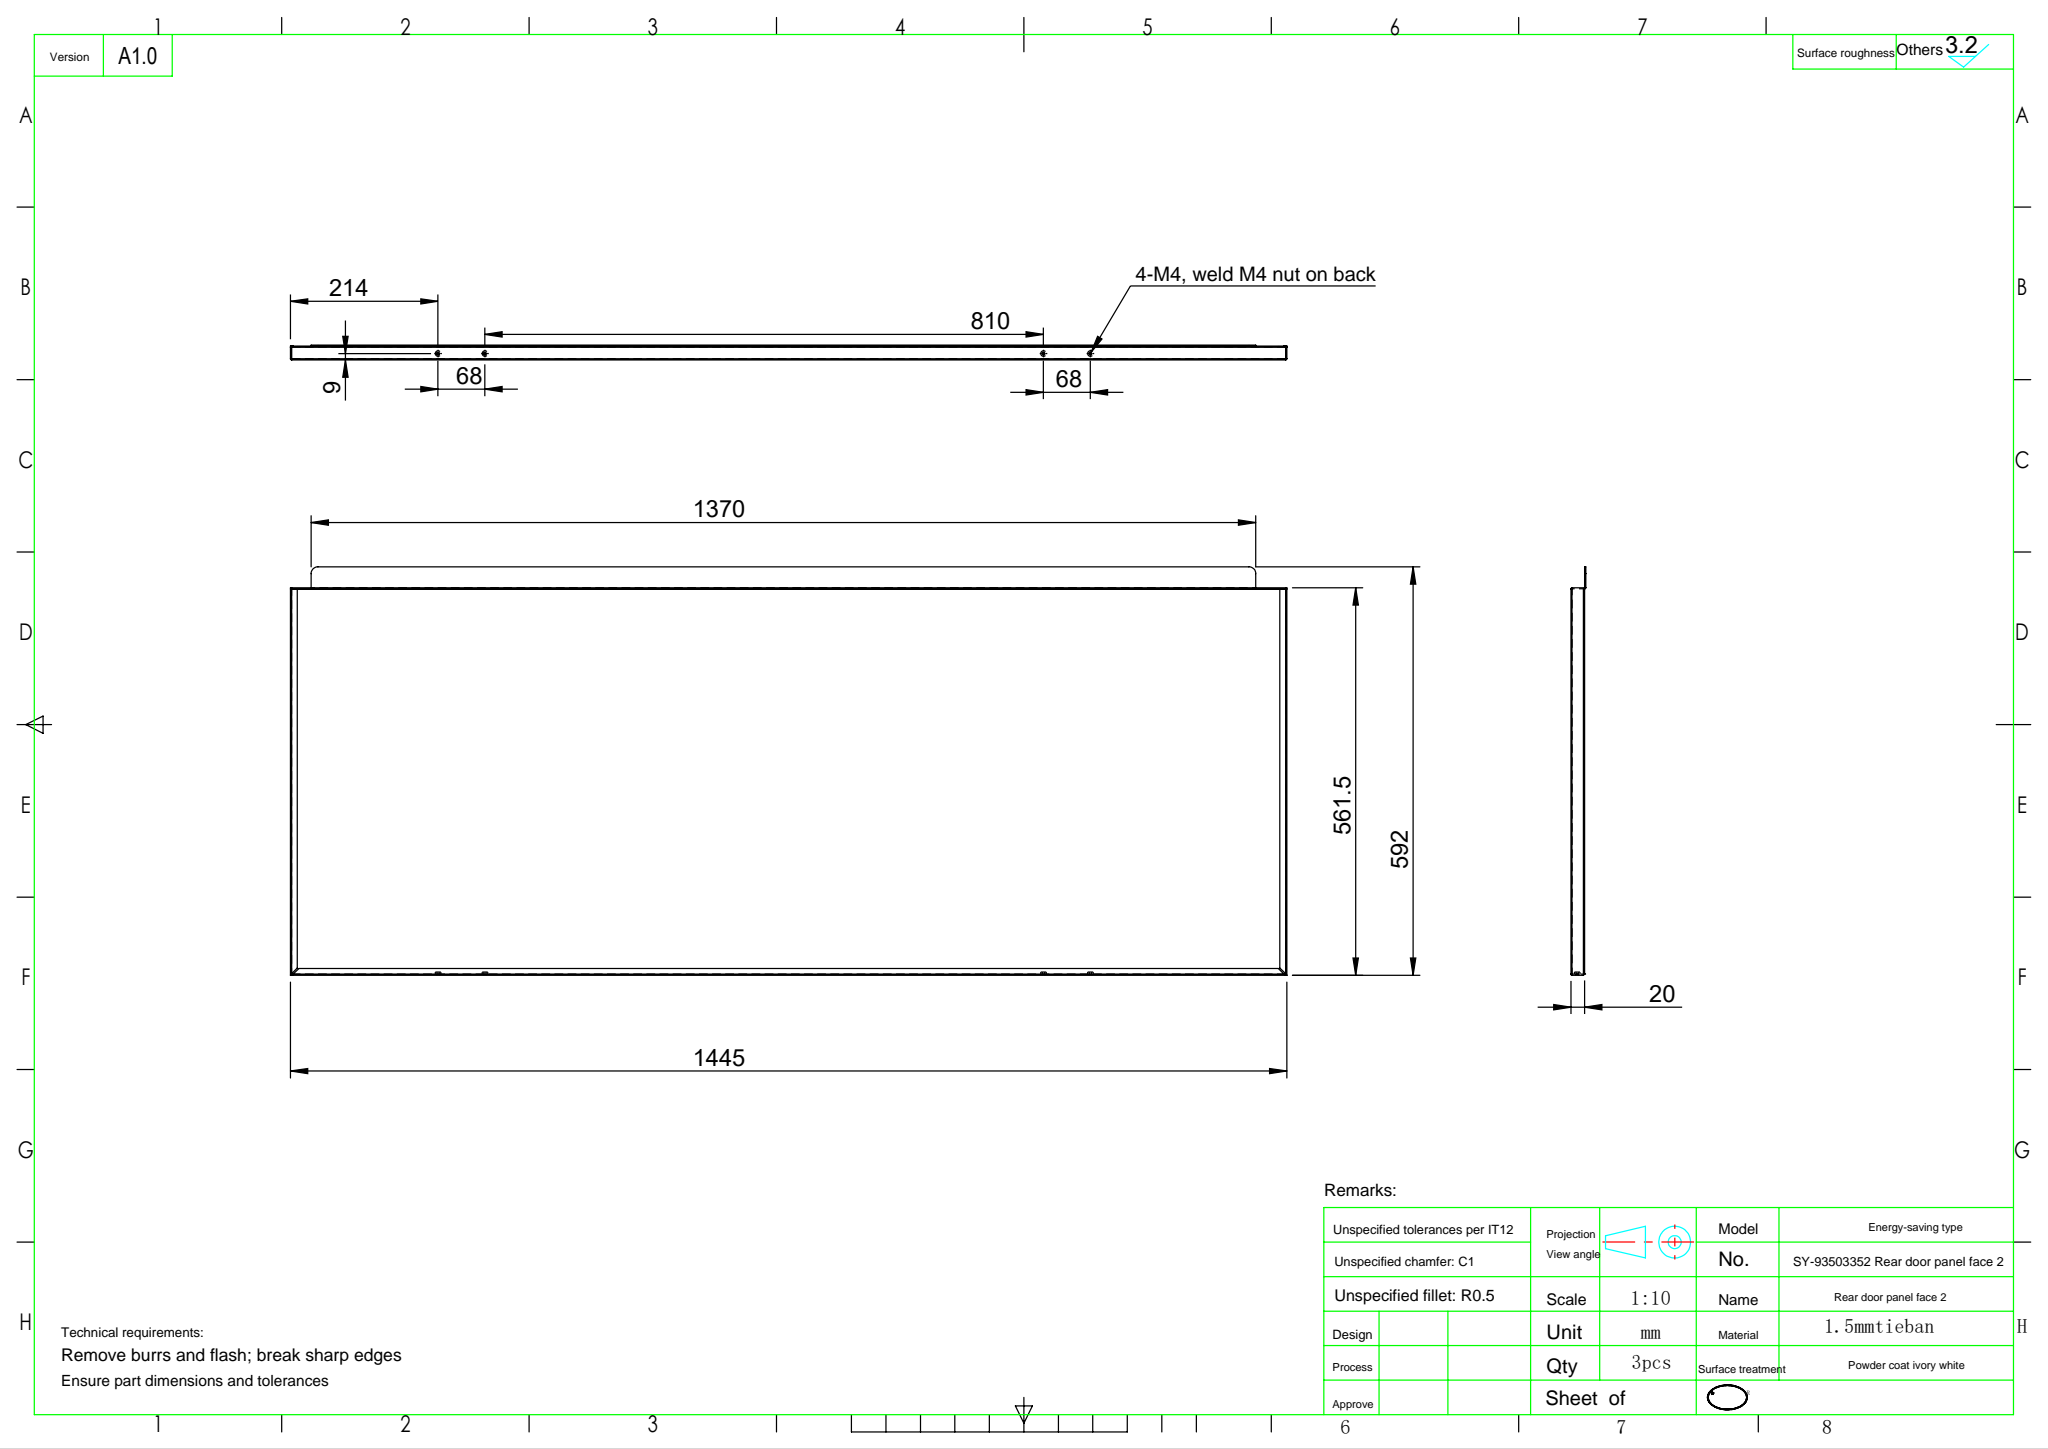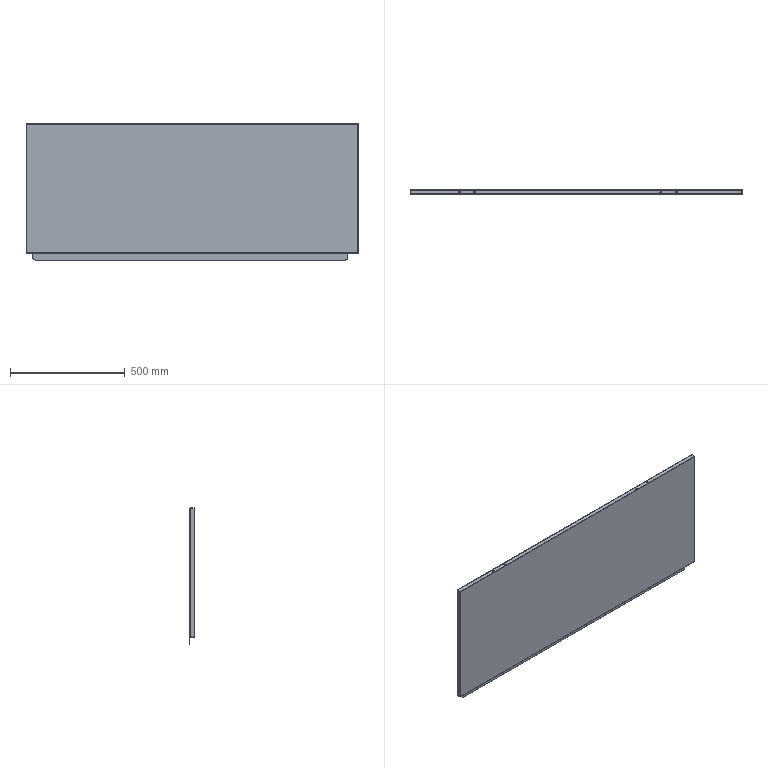Part | SolidWorks | features EdgeFlange 3, Fillet 1, FlatPattern 1, HoleWzd 1, ICE 1, SMBaseFlange 1, SheetMetal 1 | 1 solid | 120 faces | box 1445 x 21.5 x 592 mm | volume 1421822 mm3 | plane 72 | cylinder 44 | spline 4 | commonest cylinder face diameters 0.4 x8 3.2 x8 3.3 x8 3.4 x8 8 x8 0.75 x2